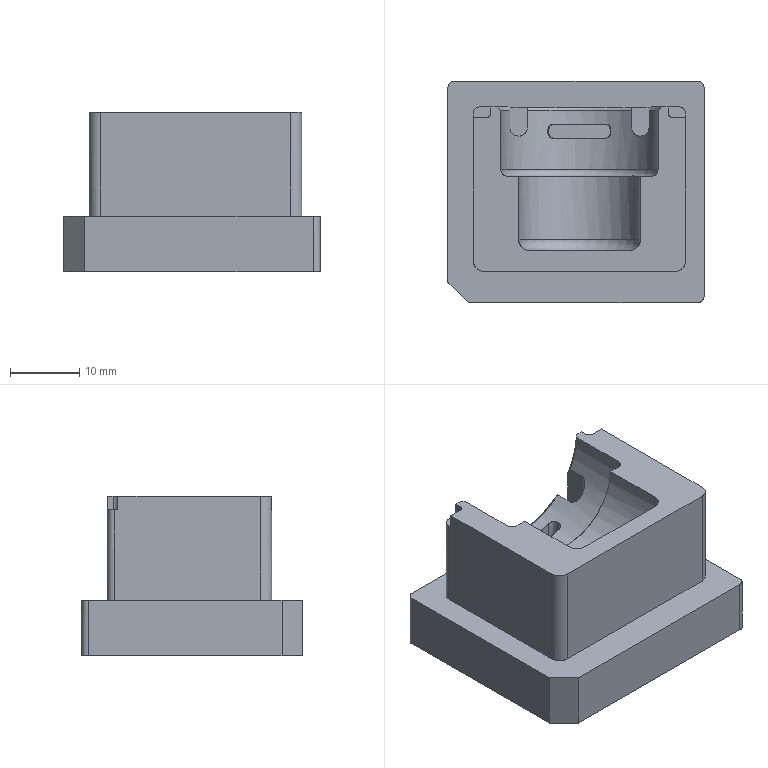NC program | PowerMill | posted with a generic post | part box 37 x 32 x 23 mm
Lines 14682 to 15635 of 159067:
N14779 M6
N14780 S20000 M03
N14781 G00 G90 X0.0 Y0.0
N14782 G43 Z9.8 H26
N14783
N14784 G05 P10000 R4
N14785 X-2.7016 Y9.3578
N14786 Z-9.56
N14787 G01 Z-10.76 F1800.0
N14788 X-2.7117 Y9.369 F3000.0
N14789 G03 X-2.904 Y9.3791 I-0.1012 J-0.0911
N14790 G01 X-3.1183 Y9.1861
N14791 X-3.3068 Y9.1312
N14792 X-3.3152 Y9.1271
N14793 X-3.3288 Y9.1186
N14794 X-3.3401 Y9.1074
N14795 X-3.3988 Y9.0345
N14796 X-3.4106 Y9.0137
N14797 X-3.4153 Y8.9902
N14798 Y8.517
N14799 X-3.4061 Y8.4613
N14800 X-3.4022 Y8.447
N14801 X-3.3955 Y8.4338
N14802 X-3.3681 Y8.3911
N14803 X-3.3281 Y8.3599
N14804 X-3.1183 Y8.2897
N14805 X-2.9128 Y8.1045
N14806 X-2.5846 Y9.3494 Z-10.8097
N14807 X-2.5965 Y9.3586
N14808 G03 X-2.7875 Y9.334 I-0.0832 J-0.1078
N14809 G01 X-2.8213 Y9.29
N14810 X-2.95 Y9.2064
N14811 X-3.1183 Y9.1551
N14812 X-3.2933 Y9.1321
N14813 X-3.3127 Y9.125
N14814 X-3.3299 Y9.1159
N14815 X-3.344 Y9.1026
N14816 X-3.3823 Y9.056
N14817 X-3.412 Y9.0036
N14818 X-3.4149 Y8.9817
N14819 X-3.4056 Y8.4701
N14820 X-3.4023 Y8.4553
N14821 X-3.3978 Y8.4416
N14822 X-3.3907 Y8.4291
N14823 X-3.3819 Y8.4167
N14824 X-3.3286 Y8.3669
N14825 X-3.3163 Y8.3576
N14826 X-3.3023 Y8.3512
N14827 X-3.2571 Y8.3361
N14828 X-3.0894 Y8.3155
N14829 X-2.8213 Y8.1827
N14830 X-2.7855 Y8.1405
N14831 X-2.4504 Y9.3033 Z-10.8594
N14832 X-2.4606 Y9.3145
N14833 G03 X-2.6529 Y9.3235 I-0.1006 J-0.0917
N14834 G01 X-2.7815 Y9.2064
N14835 X-3.1051 Y9.1591
N14836 X-3.2217 Y9.1403
N14837 X-3.3341 Y9.1043
N14838 X-3.3473 Y9.0959
N14839 X-3.3584 Y9.0848
N14840 X-3.3938 Y9.0368
N14841 X-3.4149 Y8.981
N14842 X-3.4056 Y8.4701
N14843 X-3.404 Y8.4611
N14844 X-3.4 Y8.4471
N14845 X-3.3933 Y8.4342
N14846 X-3.3867 Y8.4243
N14847 X-3.3595 Y8.3958
N14848 X-3.3287 Y8.3669
N14849 X-3.3163 Y8.3576
N14850 X-3.3023 Y8.3511
N14851 X-3.2806 Y8.3439
N14852 X-2.9315 Y8.3155
N14853 X-2.8213 Y8.2778
N14854 X-2.6713 Y8.1469
N14855 X-2.3047 Y9.2868 Z-10.9092
N14856 X-2.3163 Y9.2965
N14857 G03 X-2.5081 Y9.2795 I-0.0874 J-0.1044
N14858 G01 X-2.5243 Y9.26
N14859 X-2.613 Y9.2064
N14860 X-2.8213 Y9.1478
N14861 X-3.1183 Y9.1498
N14862 X-3.2371 Y9.1351
N14863 X-3.3135 Y9.112
N14864 X-3.331 Y9.104
N14865 X-3.3458 Y9.0916
N14866 X-3.3785 Y9.0573
N14867 X-3.4039 Y9.0174
N14868 X-3.4072 Y8.9953
N14869 X-3.408 Y8.5983
N14870 X-3.4058 Y8.4772
N14871 X-3.403 Y8.4587
N14872 X-3.3956 Y8.4416
N14873 X-3.3886 Y8.4299
N14874 X-3.345 Y8.3821
N14875 X-3.3287 Y8.3668
N14876 X-3.3164 Y8.3575
N14877 X-3.3023 Y8.3511
N14878 X-3.2999 Y8.3503
N14879 X-3.2905 Y8.3478
N14880 X-3.2809 Y8.3467
N14881 X-2.8213 Y8.3217
N14882 X-2.5243 Y8.1942
N14883 X-2.5219 Y8.1914
N14884 X-2.1548 Y9.2515 Z-10.9589
N14885 X-2.1645 Y9.2632
N14886 G03 X-2.3562 Y9.2803 I-0.1044 J-0.0874
N14887 G01 X-2.4445 Y9.2064
N14888 X-2.5243 Y9.1748
N14889 X-2.7696 Y9.1624
N14890 X-2.8213 Y9.1479
N14891 X-3.0295 Y9.1497
N14892 X-3.2372 Y9.1352
N14893 X-3.3135 Y9.112
N14894 X-3.3311 Y9.104
N14895 X-3.3458 Y9.0916
N14896 X-3.3773 Y9.0577
N14897 X-3.3991 Y9.0169
N14898 X-3.4052 Y9.0008
N14899 X-3.4073 Y8.9836
N14900 X-3.4081 Y8.5983
N14901 X-3.406 Y8.4827
N14902 X-3.4034 Y8.4648
N14903 X-3.3964 Y8.4481
N14904 X-3.392 Y8.4405
N14905 X-3.3382 Y8.3769
N14906 X-3.326 Y8.3673
N14907 X-3.3136 Y8.3595
N14908 X-3.2998 Y8.3543
N14909 X-3.2848 Y8.3504
N14910 X-2.6157 Y8.3155
N14911 X-2.5243 Y8.2868
N14912 X-2.3728 Y8.1599
N14913 X-1.9797 Y9.2832 Z-11.0086
N14914 X-1.9909 Y9.2934
N14915 G03 X-2.1832 Y9.2837 I-0.0913 J-0.101
N14916 G01 X-2.2274 Y9.2348
N14917 X-2.5243 Y9.1533
N14918 X-3.2194 Y9.1374
N14919 X-3.281 Y9.1245
N14920 X-3.3388 Y9.0994
N14921 X-3.3756 Y9.0595
N14922 X-3.3999 Y9.0109
N14923 X-3.4055 Y8.9955
N14924 X-3.4074 Y8.9792
N14925 X-3.4081 Y8.5983
N14926 X-3.406 Y8.4821
N14927 X-3.4014 Y8.458
N14928 X-3.389 Y8.4369
N14929 X-3.3561 Y8.398
N14930 X-3.3197 Y8.367
N14931 X-3.2997 Y8.3549
N14932 X-3.2768 Y8.3499
N14933 X-2.8616 Y8.3291
N14934 X-2.446 Y8.3155
N14935 X-2.2274 Y8.2182
N14936 X-2.1993 Y8.1876
N14937 X-1.8081 Y9.2431 Z-11.0584
N14938 X-1.8172 Y9.2552
N14939 G03 X-2.0079 Y9.2818 I-0.1086 J-0.0821
N14940 G01 X-2.1076 Y9.2064
N14941 X-2.2274 Y9.1641
N14942 X-2.5145 Y9.1561
N14943 X-2.5244 Y9.1534
N14944 X-3.0159 Y9.1421
N14945 X-3.225 Y9.1363
N14946 X-3.2346 Y9.1354
N14947 X-3.2439 Y9.1332
N14948 X-3.2899 Y9.1208
N14949 X-3.3326 Y9.0999
N14950 X-3.3431 Y9.0932
N14951 X-3.3522 Y9.0848
N14952 X-3.3825 Y9.0485
N14953 X-3.4006 Y9.0049
N14954 X-3.4057 Y8.9901
N14955 X-3.4074 Y8.9745
N14956 X-3.4101 Y8.7198
N14957 X-3.403 Y8.4651
N14958 X-3.3972 Y8.4495
N14959 X-3.388 Y8.4356
N14960 X-3.3695 Y8.4137
N14961 X-3.3171 Y8.3659
N14962 X-3.3082 Y8.3604
N14963 X-3.2918 Y8.3529
N14964 X-3.2741 Y8.3498
N14965 X-3.1243 Y8.3419
N14966 X-2.2539 Y8.3155
N14967 X-2.0378 Y8.1884
N14968 X-1.6422 Y9.2785 Z-11.1081
N14969 X-1.6529 Y9.289
N14970 G03 X-1.8454 Y9.2872 I-0.0954 J-0.0971
N14971 G01 X-1.9247 Y9.2064
N14972 X-2.2274 Y9.1524
N14973 X-3.2402 Y9.1344
N14974 X-3.2918 Y9.1196
N14975 X-3.339 Y9.094
N14976 X-3.3485 Y9.0875
N14977 X-3.3569 Y9.0797
N14978 X-3.3658 Y9.0699
N14979 X-3.3729 Y9.0607
N14980 X-3.3785 Y9.0506
N14981 X-3.4013 Y8.9989
N14982 X-3.4059 Y8.9848
N14983 X-3.4075 Y8.9699
N14984 X-3.4079 Y8.7092
N14985 X-3.3936 Y8.4489
N14986 X-3.3532 Y8.3983
N14987 X-3.3031 Y8.3573
N14988 X-3.273 Y8.3482
N14989 X-3.2414 Y8.348
N14990 X-2.0594 Y8.3155
N14991 X-1.9304 Y8.2684
N14992 X-1.8638 Y8.2071
N14993 X-1.4646 Y9.1594 Z-11.1578
N14994 X-1.4721 Y9.1725
N14995 G03 X-1.6576 Y9.2239 I-0.1184 J-0.067
N14996 G01 X-1.6885 Y9.2064
N14997 X-1.9304 Y9.1539
N14998 X-3.2451 Y9.133
N14999 X-3.3025 Y9.1144
N15000 X-3.3533 Y9.0816
N15001 X-3.3643 Y9.0714
N15002 X-3.373 Y9.0592
N15003 X-3.3786 Y9.0492
N15004 X-3.4075 Y8.9759
N15005 X-3.4079 Y8.7288
N15006 X-3.4001 Y8.4819
N15007 X-3.3969 Y8.4627
N15008 X-3.3887 Y8.4451
N15009 X-3.3814 Y8.4338
N15010 X-3.3447 Y8.3918
N15011 X-3.3005 Y8.3576
N15012 X-3.2721 Y8.3513
N15013 X-1.8551 Y8.3155
N15014 X-1.6744 Y8.23
N15015 X-1.2978 Y9.085 Z-11.2076
N15016 X-1.3016 Y9.0996
N15017 G03 X-1.4675 Y9.1974 I-0.1318 J-0.034
N15018 G01 X-1.6334 Y9.1545
N15019 X-2.5735 Y9.1437
N15020 X-3.2271 Y9.1333
N15021 X-3.3131 Y9.1069
N15022 X-3.3357 Y9.0932
N15023 X-3.3487 Y9.0831
N15024 X-3.3591 Y9.0704
N15025 X-3.3844 Y9.0322
N15026 X-3.402 Y8.99
N15027 X-3.4057 Y8.9774
N15028 X-3.4071 Y8.9643
N15029 X-3.4079 Y8.7327
N15030 X-3.4008 Y8.5011
N15031 X-3.3989 Y8.4868
N15032 X-3.3942 Y8.4732
N15033 X-3.3709 Y8.4228
N15034 X-3.3243 Y8.3743
N15035 X-3.3005 Y8.3576
N15036 X-3.2721 Y8.3512
N15037 X-3.0539 Y8.3457
N15038 X-1.6334 Y8.3211
N15039 X-1.4821 Y8.25
N15040 X-1.066 Y9.0829 Z-11.2573
N15041 X-1.0706 Y9.0973
N15042 G03 X-1.2418 Y9.1854 I-0.1296 J-0.0415
N15043 G01 X-1.3364 Y9.1551
N15044 X-2.8884 Y9.1388
N15045 X-3.223 Y9.1334
N15046 X-3.309 Y9.1069
N15047 X-3.3173 Y9.1038
N15048 X-3.3251 Y9.0997
N15049 X-3.3424 Y9.0892
N15050 X-3.3767 Y9.0442
N15051 X-3.4009 Y8.993
N15052 X-3.4046 Y8.9805
N15053 X-3.4059 Y8.9674
N15054 X-3.4079 Y8.7357
N15055 X-3.4009 Y8.504
N15056 X-3.399 Y8.4896
N15057 X-3.3942 Y8.4759
N15058 X-3.3588 Y8.4076
N15059 X-3.3005 Y8.3576
N15060 X-3.2535 Y8.3489
N15061 X-3.2057 Y8.3495
N15062 X-1.3246 Y8.3155
N15063 X-1.2674 Y8.2828
N15064 X-0.8021 Y9.0884 Z-11.307
N15065 X-0.8072 Y9.1026
N15066 G03 X-0.9817 Y9.1841 I-0.128 J-0.0465
N15067 G01 X-1.0394 Y9.1631
N15068 X-1.3236 Y9.1593
N15069 X-1.3364 Y9.1552
N15070 X-2.8081 Y9.1397
N15071 X-2.9688 Y9.1375
N15072 X-3.2188 Y9.1336
N15073 X-3.3131 Y9.1042
N15074 X-3.3362 Y9.0923
N15075 X-3.3539 Y9.0733
N15076 X-3.3896 Y9.018
N15077 X-3.3931 Y9.0118
N15078 X-3.3961 Y9.0054
N15079 X-3.4033 Y8.987
N15080 X-3.408 Y8.7469
N15081 X-3.401 Y8.5068
N15082 X-3.3991 Y8.4923
N15083 X-3.3943 Y8.4786
N15084 X-3.3655 Y8.4171
N15085 X-3.3287 Y8.3787
N15086 X-3.3138 Y8.3668
N15087 X-3.2963 Y8.3593
N15088 X-3.2701 Y8.3519
N15089 X-1.0593 Y8.3155
N15090 X-1.0047 Y8.2819
N15091 X-0.5582 Y9.0376 Z-11.3567
N15092 X-0.5618 Y9.0523
N15093 G03 X-0.7268 Y9.1515 I-0.1321 J-0.0329
N15094 G01 X-0.7425 Y9.1476
N15095 X-3.2162 Y9.1332
N15096 X-3.3123 Y9.1031
N15097 X-3.3352 Y9.0913
N15098 X-3.3527 Y9.0724
N15099 X-3.3913 Y9.0132
N15100 X-3.4003 Y8.9936
N15101 X-3.4034 Y8.9723
N15102 Y8.5807
N15103 X-3.4011 Y8.5068
N15104 X-3.3992 Y8.4923
N15105 X-3.3943 Y8.4786
N15106 X-3.363 Y8.4216
N15107 X-3.3184 Y8.3744
N15108 X-3.2906 Y8.3644
N15109 X-3.1987 Y8.3507
N15110 X-2.2804 Y8.3356
N15111 X-0.745 Y8.3298
N15112 X-0.335 Y8.9952 Z-11.4065
N15113 X-0.3351 Y9.0104
N15114 G03 X-0.4723 Y9.1454 I-0.1361 J-0.0011
N15115 G01 X-3.2472 Y9.1235
N15116 X-3.3012 Y9.1066
N15117 X-3.3573 Y9.0654
N15118 X-3.3872 Y9.0195
N15119 X-3.4034 Y8.9462
N15120 X-3.4032 Y8.7167
N15121 X-3.3925 Y8.4875
N15122 X-3.3905 Y8.4735
N15123 X-3.3858 Y8.4602
N15124 X-3.3815 Y8.4511
N15125 X-3.3402 Y8.3943
N15126 X-3.3289 Y8.3841
N15127 X-3.3168 Y8.3753
N15128 X-3.303 Y8.3691
N15129 X-3.2938 Y8.366
N15130 X-3.1907 Y8.3505
N15131 X-2.3656 Y8.3369
N15132 X-0.4795 Y8.3302
N15133 G00 Z-0.5079
N15134 G01 X-8.6977 Y9.5965 F10000.0
N15135 G00 Z-6.4269
N15136 G01 Z-7.6269 F1800.0
N15137 X-8.7203 Y9.5963 F3000.0
N15138 G03 X-8.9222 Y9.3917 I0.0014 J-0.2032
N15139 G01 X-8.9218 Y9.3433
N15140 X-8.91 Y9.181
N15141 X-8.896 Y9.1401
N15142 X-8.8245 Y8.9486
N15143 X-8.8209 Y8.9406
N15144 X-8.8163 Y8.933
N15145 X-8.7892 Y8.8936
N15146 X-8.7813 Y8.884
N15147 X-8.7719 Y8.8759
N15148 X-8.5719 Y8.7323
N15149 X-8.5572 Y8.7232
N15150 X-8.5504 Y8.7194
N15151 X-8.5432 Y8.7164
N15152 X-8.4303 Y8.6762
N15153 X-8.3054 Y8.6764
N15154 X-8.6832 Y9.6252 Z-7.6767
N15155 X-8.7058 Y9.6267
N15156 G03 X-8.9225 Y9.438 I-0.014 J-0.2027
N15157 G01 X-8.9209 Y9.2871
N15158 X-8.8954 Y9.1383
N15159 X-8.8245 Y8.9486
N15160 X-8.8209 Y8.9405
N15161 X-8.8164 Y8.933
N15162 X-8.7892 Y8.8935
N15163 X-8.7813 Y8.8839
N15164 X-8.7719 Y8.8758
N15165 X-8.5719 Y8.7323
N15166 X-8.5572 Y8.7232
N15167 X-8.5504 Y8.7194
N15168 X-8.5433 Y8.7164
N15169 X-8.4421 Y8.6804
N15170 X-8.4302 Y8.6772
N15171 X-8.4179 Y8.6762
N15172 X-8.2565 Y8.6764
N15173 X-8.6833 Y9.6449 Z-7.7264
N15174 X-8.7059 Y9.6465
N15175 G03 X-8.9227 Y9.4578 I-0.0141 J-0.2027
N15176 G01 X-8.9213 Y9.2961
N15177 X-8.8948 Y9.1365
N15178 X-8.8246 Y8.9486
N15179 X-8.821 Y8.9405
N15180 X-8.8164 Y8.933
N15181 X-8.7893 Y8.8935
N15182 X-8.7814 Y8.8839
N15183 X-8.7719 Y8.8758
N15184 X-8.5719 Y8.7323
N15185 X-8.5573 Y8.7231
N15186 X-8.5505 Y8.7194
N15187 X-8.5433 Y8.7164
N15188 X-8.4421 Y8.6803
N15189 X-8.4302 Y8.6772
N15190 X-8.4179 Y8.6761
N15191 X-8.0968 Y8.6765
N15192 X-8.0488 Y8.6839
N15193 X-8.6924 Y9.6782 Z-7.7761
N15194 X-8.7149 Y9.6787
N15195 G03 X-8.9229 Y9.4803 I-0.0048 J-0.2032
N15196 G01 X-8.9215 Y9.3307
N15197 X-8.9102 Y9.1816
N15198 X-8.8942 Y9.1348
N15199 X-8.8246 Y8.9486
N15200 X-8.821 Y8.9405
N15201 X-8.8165 Y8.933
N15202 X-8.7893 Y8.8935
N15203 X-8.7814 Y8.8839
N15204 X-8.772 Y8.8758
N15205 X-8.5719 Y8.7322
N15206 X-8.5573 Y8.7231
N15207 X-8.5505 Y8.7193
N15208 X-8.5433 Y8.7163
N15209 X-8.4421 Y8.6803
N15210 X-8.4302 Y8.6771
N15211 X-8.4179 Y8.6761
N15212 X-8.116 Y8.6764
N15213 X-7.9939 Y8.701
N15214 X-8.6921 Y9.7007 Z-7.8259
N15215 X-8.7146 Y9.7013
N15216 G03 X-8.9231 Y9.5034 I-0.0053 J-0.2032
N15217 G01 X-8.922 Y9.3424
N15218 X-8.9103 Y9.1818
N15219 X-8.8936 Y9.133
N15220 X-8.8247 Y8.9486
N15221 X-8.8211 Y8.9405
N15222 X-8.8165 Y8.9329
N15223 X-8.7894 Y8.8934
N15224 X-8.7815 Y8.8839
N15225 X-8.772 Y8.8758
N15226 X-8.572 Y8.7322
N15227 X-8.5573 Y8.723
N15228 X-8.5505 Y8.7193
N15229 X-8.5433 Y8.7163
N15230 X-8.4421 Y8.6802
N15231 X-8.4302 Y8.6771
N15232 X-8.4179 Y8.6761
N15233 X-8.1279 Y8.6764
N15234 X-7.9264 Y8.7265
N15235 X-8.6918 Y9.7256 Z-7.8756
N15236 X-8.7144 Y9.7262
N15237 G03 X-8.9233 Y9.5288 I-0.0058 J-0.2032
N15238 G01 X-8.9226 Y9.3552
N15239 X-8.9103 Y9.182
N15240 X-8.893 Y9.1312
N15241 X-8.8247 Y8.9485
N15242 X-8.8211 Y8.9405
N15243 X-8.8166 Y8.9329
N15244 X-8.7894 Y8.8934
N15245 X-8.7815 Y8.8838
N15246 X-8.7721 Y8.8757
N15247 X-8.572 Y8.7321
N15248 X-8.5573 Y8.723
N15249 X-8.5505 Y8.7192
N15250 X-8.5434 Y8.7162
N15251 X-8.4422 Y8.6802
N15252 X-8.4302 Y8.677
N15253 X-8.4179 Y8.676
N15254 X-8.1352 Y8.6763
N15255 X-7.9021 Y8.7437
N15256 X-8.6916 Y9.7554 Z-7.9253
N15257 X-8.7141 Y9.7561
N15258 G03 X-8.9236 Y9.5593 I-0.0063 J-0.2031
N15259 G01 X-8.9232 Y9.3705
N15260 X-8.9104 Y9.1822
N15261 X-8.8923 Y9.1295
N15262 X-8.8248 Y8.9485
N15263 X-8.8212 Y8.9405
N15264 X-8.8166 Y8.9329
N15265 X-8.7894 Y8.8934
N15266 X-8.7815 Y8.8838
N15267 X-8.7721 Y8.8757
N15268 X-8.572 Y8.7321
N15269 X-8.5574 Y8.7229
N15270 X-8.5506 Y8.7192
N15271 X-8.5434 Y8.7162
N15272 X-8.4322 Y8.6766
N15273 X-8.4141 Y8.676
N15274 X-8.1404 Y8.6762
N15275 X-7.8743 Y8.7632
N15276 X-8.7682 Y9.7217 Z-7.975
N15277 X-8.7833 Y9.7222
N15278 G03 X-8.9239 Y9.5907 I-0.0045 J-0.136
N15279 G01 Y9.3863
N15280 X-8.9105 Y9.1823
N15281 X-8.8917 Y9.1277
N15282 X-8.8248 Y8.9485
N15283 X-8.8212 Y8.9404
N15284 X-8.8167 Y8.9329
N15285 X-8.7895 Y8.8934
N15286 X-8.7816 Y8.8838
N15287 X-8.7722 Y8.8757
N15288 X-8.5721 Y8.732
N15289 X-8.5574 Y8.7229
N15290 X-8.5506 Y8.7191
N15291 X-8.5434 Y8.7161
N15292 X-8.4332 Y8.6769
N15293 X-8.4044 Y8.6759
N15294 X-8.1441 Y8.6762
N15295 X-7.87 Y8.7739
N15296 X-7.8367 Y8.7771
N15297 X-8.7738 Y9.7672 Z-8.0248
N15298 X-8.789 Y9.7671
N15299 G03 X-8.9242 Y9.6301 I0.001 J-0.1361
N15300 G01 X-8.9222 Y9.3433
N15301 X-8.9105 Y9.1825
N15302 X-8.8911 Y9.1259
N15303 X-8.8249 Y8.9485
N15304 X-8.8213 Y8.9404
N15305 X-8.8167 Y8.9329
N15306 X-8.7895 Y8.8933
N15307 X-8.7816 Y8.8837
N15308 X-8.7722 Y8.8756
N15309 X-8.5721 Y8.732
N15310 X-8.5574 Y8.7229
N15311 X-8.5506 Y8.7191
N15312 X-8.5435 Y8.7161
N15313 X-8.4342 Y8.6772
N15314 X-8.3942 Y8.6759
N15315 X-8.1565 Y8.6761
N15316 X-8.1443 Y8.6772
N15317 X-8.1324 Y8.6803
N15318 X-7.9288 Y8.7529
N15319 X-7.87 Y8.7831
N15320 X-7.7946 Y8.7963
N15321 X-8.7741 Y9.8053 Z-8.0745
N15322 X-8.7893 Y9.8052
N15323 G03 X-8.9245 Y9.6682 I0.0009 J-0.1361
N15324 G01 X-8.9223 Y9.3433
N15325 X-8.9106 Y9.1827
N15326 X-8.8905 Y9.1242
N15327 X-8.8249 Y8.9485
N15328 X-8.8213 Y8.9404
N15329 X-8.8168 Y8.9329
N15330 X-8.7896 Y8.8933
N15331 X-8.7817 Y8.8837
N15332 X-8.7722 Y8.8756
N15333 X-8.5721 Y8.732
N15334 X-8.5574 Y8.7228
N15335 X-8.5506 Y8.7191
N15336 X-8.5435 Y8.7161
N15337 X-8.4352 Y8.6775
N15338 X-8.3835 Y8.6758
N15339 X-8.1565 Y8.6761
N15340 X-8.1443 Y8.6771
N15341 X-8.1324 Y8.6803
N15342 X-7.9473 Y8.7462
N15343 X-7.87 Y8.7894
N15344 X-7.7321 Y8.826
N15345 X-8.7744 Y9.835 Z-8.1242
N15346 X-8.7895 Y9.8349
N15347 G03 X-8.9247 Y9.6978 I0.0009 J-0.1362
N15348 G01 X-8.9223 Y9.3433
N15349 X-8.9107 Y9.1829
N15350 X-8.8899 Y9.1224
N15351 X-8.8249 Y8.9484
N15352 X-8.8214 Y8.9404
N15353 X-8.8168 Y8.9328
N15354 X-8.7896 Y8.8933
N15355 X-8.7817 Y8.8837
N15356 X-8.7723 Y8.8756
N15357 X-8.5721 Y8.7319
N15358 X-8.5575 Y8.7228
N15359 X-8.5507 Y8.719
N15360 X-8.5435 Y8.716
N15361 X-8.4497 Y8.6826
N15362 X-8.3032 Y8.6758
N15363 X-8.1565 Y8.676
N15364 X-8.1443 Y8.6771
N15365 X-8.1324 Y8.6802
N15366 X-7.9574 Y8.7426
N15367 X-7.87 Y8.7946
N15368 X-7.6678 Y8.8672
N15369 X-8.7746 Y9.8586 Z-8.174
N15370 X-8.7897 Y9.8585
N15371 G03 X-8.9249 Y9.7214 I0.0009 J-0.1362
N15372 G01 X-8.9224 Y9.3433
N15373 X-8.9107 Y9.1831
N15374 X-8.8893 Y9.1206
N15375 X-8.825 Y8.9484
N15376 X-8.8214 Y8.9404
N15377 X-8.8169 Y8.9328
N15378 X-8.7897 Y8.8933
N15379 X-8.7818 Y8.8837
N15380 X-8.7723 Y8.8756
N15381 X-8.5722 Y8.7319
N15382 X-8.5575 Y8.7227
N15383 X-8.5507 Y8.719
N15384 X-8.5435 Y8.716
N15385 X-8.4501 Y8.6827
N15386 X-8.3034 Y8.6759
N15387 X-8.1565 Y8.676
N15388 X-8.1443 Y8.677
N15389 X-8.1324 Y8.6802
N15390 X-7.9574 Y8.7425
N15391 X-7.87 Y8.7946
N15392 X-7.8633 Y8.797
N15393 X-7.6714 Y8.9095
N15394 X-7.6386 Y8.9178
N15395 X-8.7748 Y9.8839 Z-8.2237
N15396 X-8.7899 Y9.8838
N15397 G03 X-8.9252 Y9.7467 I0.0009 J-0.1361
N15398 G01 X-8.9224 Y9.3433
N15399 X-8.9108 Y9.1833
N15400 X-8.8887 Y9.1188
N15401 X-8.825 Y8.9484
N15402 X-8.8215 Y8.9404
N15403 X-8.8169 Y8.9328
N15404 X-8.7897 Y8.8932
N15405 X-8.7818 Y8.8836
N15406 X-8.7724 Y8.8755
N15407 X-8.5722 Y8.7318
N15408 X-8.5575 Y8.7227
N15409 X-8.5507 Y8.7189
N15410 X-8.5436 Y8.7159
N15411 X-8.4505 Y8.6828
N15412 X-8.3036 Y8.676
N15413 X-8.1565 Y8.6759
N15414 X-8.1443 Y8.677
N15415 X-8.1324 Y8.6801
N15416 X-7.9714 Y8.7375
N15417 X-7.7215 Y8.9095
N15418 X-7.5971 Y8.9594
N15419 X-8.7751 Y9.9137 Z-8.2734
N15420 X-8.7902 Y9.9136
N15421 G03 X-8.9254 Y9.7765 I0.0009 J-0.1362
N15422 G01 X-8.9225 Y9.3433
N15423 X-8.9109 Y9.1835
N15424 X-8.8881 Y9.1171
N15425 X-8.8251 Y8.9484
N15426 X-8.8215 Y8.9403
N15427 X-8.817 Y8.9328
N15428 X-8.7897 Y8.8932
N15429 X-8.7818 Y8.8836
N15430 X-8.7724 Y8.8755
N15431 X-8.5722 Y8.7318
N15432 X-8.5576 Y8.7226
N15433 X-8.5508 Y8.7189
N15434 X-8.5436 Y8.7159
N15435 X-8.4509 Y8.6829
N15436 X-8.3038 Y8.6761
N15437 X-8.1565 Y8.6759
N15438 X-8.1443 Y8.6769
N15439 X-8.1324 Y8.6801
N15440 X-7.9803 Y8.7343
N15441 X-7.9717 Y8.738
N15442 X-7.9636 Y8.7428
N15443 X-7.8205 Y8.8413
N15444 X-7.7454 Y8.9095
N15445 X-7.573 Y9.0042
N15446 X-7.5422 Y9.0072
N15447 X-8.7753 Y9.9453 Z-8.3232
N15448 X-8.7905 Y9.9452
N15449 G03 X-8.9257 Y9.8081 I0.001 J-0.1362
N15450 G01 X-8.9225 Y9.3433
N15451 X-8.9109 Y9.1837
N15452 X-8.8875 Y9.1153
N15453 X-8.8251 Y8.9484
N15454 X-8.8215 Y8.9403
N15455 X-8.817 Y8.9328
N15456 X-8.7898 Y8.8932
N15457 X-8.7819 Y8.8836
N15458 X-8.7724 Y8.8755
N15459 X-8.5722 Y8.7318
N15460 X-8.5576 Y8.7226
N15461 X-8.5508 Y8.7188
N15462 X-8.5436 Y8.7159
N15463 X-8.4513 Y8.6829
N15464 X-8.2925 Y8.6756
N15465 X-8.1336 Y8.6796
N15466 X-7.9803 Y8.7342
N15467 X-7.9717 Y8.7379
N15468 X-7.9636 Y8.7427
N15469 X-7.8384 Y8.8289
N15470 X-7.76 Y8.9095
N15471 X-7.573 Y9.0439
N15472 X-7.5109 Y9.0552
N15473 X-8.7756 Y9.984 Z-8.3729
N15474 X-8.7908 Y9.9839
N15475 G03 X-8.926 Y9.8468 I0.001 J-0.1361
N15476 G01 X-8.9226 Y9.3433
N15477 X-8.911 Y9.1839
N15478 X-8.8869 Y9.1136
N15479 X-8.8252 Y8.9484
N15480 X-8.8216 Y8.9403
N15481 X-8.8171 Y8.9328
N15482 X-8.7898 Y8.8931
N15483 X-8.7819 Y8.8835
N15484 X-8.7725 Y8.8754
N15485 X-8.5723 Y8.7317
N15486 X-8.5576 Y8.7226
N15487 X-8.5508 Y8.7188
N15488 X-8.5436 Y8.7158
N15489 X-8.4615 Y8.6865
N15490 X-8.4511 Y8.6837
N15491 X-8.4404 Y8.6824
N15492 X-8.2853 Y8.6757
N15493 X-8.13 Y8.6808
N15494 X-7.9802 Y8.7342
N15495 X-7.9716 Y8.7379
N15496 X-7.9636 Y8.7427
N15497 X-7.8384 Y8.8288
N15498 X-7.76 Y8.9094
N15499 X-7.7336 Y8.9284
N15500 X-7.573 Y9.0837
N15501 X-7.4663 Y9.1139
N15502 X-8.7761 Y10.0381 Z-8.4226
N15503 X-8.7912 Y10.038
N15504 G03 X-8.9264 Y9.9009 I0.0009 J-0.1362
N15505 G01 X-8.9226 Y9.3433
N15506 X-8.911 Y9.1841
N15507 X-8.8863 Y9.1118
N15508 X-8.8252 Y8.9483
N15509 X-8.8216 Y8.9403
N15510 X-8.8171 Y8.9327
N15511 X-8.7899 Y8.8931
N15512 X-8.782 Y8.8835
N15513 X-8.7725 Y8.8754
N15514 X-8.5723 Y8.7317
N15515 X-8.5576 Y8.7225
N15516 X-8.5508 Y8.7188
N15517 X-8.5437 Y8.7158
N15518 X-8.4513 Y8.6829
N15519 X-8.2889 Y8.675
N15520 X-8.1265 Y8.682
N15521 X-7.9802 Y8.7341
N15522 X-7.9716 Y8.7378
N15523 X-7.9636 Y8.7426
N15524 X-7.8465 Y8.8232
N15525 X-7.573 Y9.1325
N15526 X-7.4531 Y9.1968
N15527 X-8.7764 Y10.0863 Z-8.4724
N15528 X-8.7915 Y10.0862
N15529 G03 X-8.9268 Y9.9492 I0.0009 J-0.1361
N15530 G01 X-8.9227 Y9.3433
N15531 X-8.9111 Y9.1843
N15532 X-8.8857 Y9.11
N15533 X-8.8253 Y8.9483
N15534 X-8.8217 Y8.9403
N15535 X-8.8172 Y8.9327
N15536 X-8.7899 Y8.8931
N15537 X-8.782 Y8.8835
N15538 X-8.7726 Y8.8754
N15539 X-8.5723 Y8.7316
N15540 X-8.5577 Y8.7225
N15541 X-8.5509 Y8.7187
N15542 X-8.5437 Y8.7157
N15543 X-8.4517 Y8.6829
N15544 X-8.263 Y8.6756
N15545 X-8.152 Y8.6757
N15546 X-8.1231 Y8.6832
N15547 X-7.9802 Y8.7341
N15548 X-7.9716 Y8.7378
N15549 X-7.9636 Y8.7426
N15550 X-7.854 Y8.818
N15551 X-7.573 Y9.1914
N15552 X-7.4236 Y9.2671
N15553 X-8.7769 Y10.1466 Z-8.5221
N15554 X-8.792 Y10.1465
N15555 G03 X-8.9272 Y10.0094 I0.0009 J-0.1361
N15556 G01 X-8.9227 Y9.3433
N15557 X-8.9112 Y9.1844
N15558 X-8.8851 Y9.1082
N15559 X-8.8253 Y8.9483
N15560 X-8.8217 Y8.9403
N15561 X-8.8172 Y8.9327
N15562 X-8.7899 Y8.8931
N15563 X-8.782 Y8.8835
N15564 X-8.7726 Y8.8754
N15565 X-8.5724 Y8.7316
N15566 X-8.5577 Y8.7224
N15567 X-8.5509 Y8.7187
N15568 X-8.5437 Y8.7157
N15569 X-8.4522 Y8.6831
N15570 X-8.2552 Y8.6755
N15571 X-8.1535 Y8.6756
N15572 X-8.1198 Y8.6843
N15573 X-7.9802 Y8.734
N15574 X-7.9716 Y8.7377
N15575 X-7.9635 Y8.7425
N15576 X-7.8637 Y8.8113
N15577 X-7.8547 Y8.8186
N15578 X-7.847 Y8.8273
N15579 X-7.7234 Y8.9915
N15580 X-7.573 Y9.2727
N15581 X-7.4285 Y9.3692
N15582 X-8.7775 Y10.2291 Z-8.5718
N15583 X-8.7926 Y10.229
N15584 G03 X-8.9278 Y10.092 I0.0009 J-0.1361
N15585 G01 X-8.9228 Y9.3433
N15586 X-8.9112 Y9.1846
N15587 X-8.8844 Y9.1064
N15588 X-8.8254 Y8.9483
N15589 X-8.8218 Y8.9402
N15590 X-8.8172 Y8.9327
N15591 X-8.79 Y8.893
N15592 X-8.7821 Y8.8834
N15593 X-8.7726 Y8.8753
N15594 X-8.5724 Y8.7316
N15595 X-8.5577 Y8.7224
N15596 X-8.5509 Y8.7186
N15597 X-8.5437 Y8.7156
N15598 X-8.4532 Y8.6834
N15599 X-8.2435 Y8.6755
N15600 X-8.1554 Y8.6756
N15601 X-8.1155 Y8.6858
N15602 X-7.9802 Y8.734
N15603 X-7.9716 Y8.7377
N15604 X-7.9635 Y8.7425
N15605 X-7.8637 Y8.8112
N15606 X-7.8546 Y8.8186
N15607 X-7.8469 Y8.8272
N15608 X-7.7286 Y8.9845
N15609 X-7.6942 Y9.0495
N15610 X-7.6609 Y9.2064
N15611 X-7.6607 Y9.5448
N15612 X-8.7783 Y10.339 Z-8.6215
N15613 X-8.7934 Y10.3389
N15614 G03 X-8.9286 Y10.2019 I0.0009 J-0.1361
N15615 G01 X-8.9228 Y9.3433
N15616 X-8.9113 Y9.1848
N15617 X-8.8838 Y9.1047
N15618 X-8.8254 Y8.9483
N15619 X-8.8218 Y8.9402
N15620 X-8.8173 Y8.9327
N15621 X-8.79 Y8.893
N15622 X-8.7821 Y8.8834
N15623 X-8.7727 Y8.8753
N15624 X-8.5724 Y8.7315
N15625 X-8.5577 Y8.7223
N15626 X-8.5509 Y8.7186
N15627 X-8.5438 Y8.7156
N15628 X-8.4537 Y8.6835
N15629 X-8.2375 Y8.6754
N15630 X-8.1564 Y8.6755
N15631 X-8.1133 Y8.6865
N15632 X-7.9802 Y8.7339
N15633 X-7.9716 Y8.7376
N15634 X-7.9635 Y8.7424
N15635 X-7.8636 Y8.8112
N15636 X-7.8546 Y8.8185
N15637 X-7.8469 Y8.8272
N15638 X-7.7303 Y8.9822
N15639 X-7.6946 Y9.0495
N15640 X-7.6614 Y9.2064
N15641 X-7.661 Y9.6625
N15642 G00 Z-0.2933
N15643 G01 X-9.0593 Y12.838 F10000.0
N15644 G00 Z-7.4713
N15645 G01 Z-8.6713 F1800.0
N15646 X-9.0697 Y12.827 F3000.0
N15647 G03 X-9.0639 Y12.6346 I0.0991 J-0.0933
N15648 G01 X-9.058 Y12.629
N15649 X-8.9719 Y12.4732
N15650 X-8.9321 Y12.1763
N15651 X-8.9322 Y10.7598
N15652 X-8.9229 Y9.3433
N15653 X-8.9114 Y9.185
N15654 X-8.8832 Y9.1029
N15655 X-8.8255 Y8.9482
N15656 X-8.8219 Y8.9402
N15657 X-8.8173 Y8.9327
N15658 X-8.7901 Y8.893
N15659 X-8.7822 Y8.8834
N15660 X-8.7727 Y8.8753
N15661 X-8.5724 Y8.7315
N15662 X-8.5578 Y8.7223
N15663 X-8.551 Y8.7186
N15664 X-8.5438 Y8.7156
N15665 X-8.4545 Y8.6837
N15666 X-8.2283 Y8.6754
N15667 X-8.1685 Y8.6741
N15668 X-8.1102 Y8.6875
N15669 X-7.9801 Y8.7339
N15670 X-7.9715 Y8.7376
N15671 X-7.9635 Y8.7424
N15672 X-7.8636 Y8.8111
N15673 X-7.8546 Y8.8185
N15674 X-7.8469 Y8.8272
N15675 X-7.7302 Y8.9822
N15676 X-7.7186 Y9.0042
N15677 X-7.6622 Y9.2064
N15678 X-7.6608 Y9.9075
N15679 X-7.6595 Y11.5823
N15680 X-7.6572 Y11.6713
N15681 X-7.6568 Y11.8793
N15682 X-7.573 Y12.1415
N15683 X-7.3425 Y12.3412
N15684 X-9.0602 Y12.8388 Z-8.721
N15685 X-9.0705 Y12.8278
N15686 G03 X-9.0647 Y12.6354 I0.0991 J-0.0933
N15687 G01 X-9.058 Y12.629
N15688 X-8.9719 Y12.4732
N15689 X-8.9321 Y12.1763
N15690 X-8.9323 Y10.7598
N15691 X-8.9229 Y9.3433
N15692 X-8.9114 Y9.1852
N15693 X-8.8826 Y9.1012
N15694 X-8.8255 Y8.9482
N15695 X-8.8219 Y8.9402
N15696 X-8.8174 Y8.9326
N15697 X-8.7901 Y8.8929
N15698 X-8.7822 Y8.8833
N15699 X-8.7728 Y8.8752
N15700 X-8.5725 Y8.7314
N15701 X-8.5578 Y8.7223
N15702 X-8.551 Y8.7185
N15703 X-8.5438 Y8.7155
N15704 X-8.4553 Y8.684
N15705 X-8.2184 Y8.6754
N15706 X-8.1616 Y8.6751
N15707 X-8.1065 Y8.6888
N15708 X-7.9801 Y8.7338
N15709 X-7.9715 Y8.7376
N15710 X-7.9635 Y8.7424
N15711 X-7.8636 Y8.8111
N15712 X-7.8546 Y8.8184
N15713 X-7.8469 Y8.8271
N15714 X-7.7302 Y8.9821
N15715 X-7.7193 Y9.0027
N15716 X-7.663 Y9.2064
N15717 X-7.662 Y9.2956
N15718 X-7.6607 Y9.9075
N15719 X-7.6594 Y11.5823
N15720 X-7.6592 Y11.5906
N15721 Y11.8793
N15722 X-7.5747 Y12.1763
N15723 X-7.3461 Y12.3755
N15724 X-9.0716 Y12.8496 Z-8.7708
N15725 X-9.082 Y12.8386
N15726 G03 X-9.0762 Y12.6462 I0.0991 J-0.0933
N15727 G01 X-9.058 Y12.629
N15728 X-8.9719 Y12.4732
N15729 X-8.9321 Y12.1763
N15730 X-8.9323 Y10.7598
N15731 X-8.923 Y9.3433
N15732 X-8.9115 Y9.1854